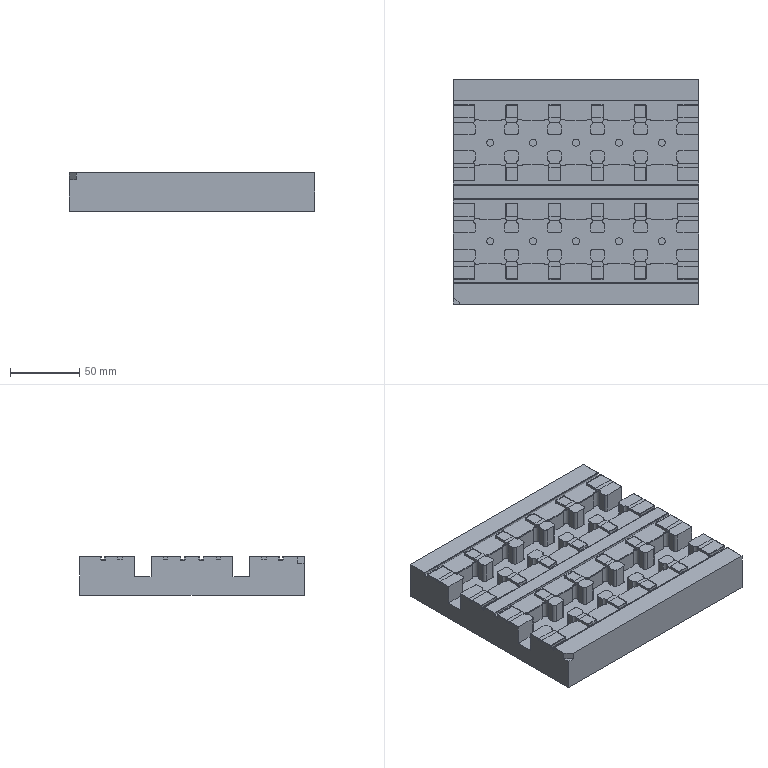NC program | NX | posted by the shop | part box 177 x 162 x 28 mm
Lines 617 to 1664 of 254847:
N4 T10 M06
(D10  D=10. R=0. H=10 ce=0.15 di=0.06)
(MAX_Z=43. MIN_Z=13.56 Time=62.88M)
T05
G00 G90 G54 X96.65 Y35.6 M03 S3000
G43 H10 Z40.
M08
Z29.302
G01 Z27.802 F2000.
X93.4
Y34.75
X74.25
G03 X67.1 Y27.6 I0.0 J-7.15
G01 Y24.98
X56.9
Y27.6
G03 X49.75 Y34.75 I-7.15 J0.0
G01 X43.25
G03 X36.1 Y27.6 I0.0 J-7.15
G01 Y24.98
X25.9
Y27.6
G03 X18.75 Y34.75 I-7.15 J0.0
G01 X12.25
G03 X5.1 Y27.6 I0.0 J-7.15
G01 Y24.98
X-5.1
Y27.6
G03 X-12.25 Y34.75 I-7.15 J0.0
G01 X-18.75
G03 X-25.9 Y27.6 I0.0 J-7.15
G01 Y24.98
X-36.1
Y27.6
G03 X-43.25 Y34.75 I-7.15 J0.0
G01 X-49.75
G03 X-56.9 Y27.6 I0.0 J-7.15
G01 Y24.98
X-67.1
Y27.6
G03 X-74.25 Y34.75 I-7.15 J0.0
G01 X-93.4
Y36.45
X-74.25
G03 X-67.1 Y43.6 I0.0 J7.15
G01 Y46.22
X-56.9
Y43.6
G03 X-55.287 Y39.077 I7.15 J0.0
G02 X-55.062 Y38.444 I-.774 J-.633
X-55.402 Y37.693 I-1. J0.0
G01 X-59.214 Y34.344
G03 X-59.38 Y34.156 I.66 J-.751
X-61.111 Y30.178 I9.63 J-6.556
G02 X-61.989 Y29.479 I-.877 J.202
G01 X-62.015 Y29.48
G02 X-62.889 Y30.178 I.003 J.9
G03 X-65.227 Y34.97 I-11.361 J-2.578
G02 X-65.451 Y35.6 I.777 J.63
X-65.227 Y36.23 I1. J0.0
G03 X-62.889 Y41.022 I-9.023 J7.37
G02 X-62.011 Y41.721 I.877 J-.202
G01 X-61.985 Y41.72
G02 X-61.111 Y41.022 I-.003 J-.9
G03 X-60.428 Y38.941 I11.361 J2.578
X-59.511 Y38.341 I.916 J.4
X-59.177 Y38.398 I0.0 J1.
G01 X-56.397 Y39.386
G02 X-56.062 Y39.444 I.335 J-.942
X-55.287 Y39.077 I0.0 J-1.
G03 X-49.75 Y36.45 I5.537 J4.523
G01 X-43.25
G03 X-36.1 Y43.6 I0.0 J7.15
G01 Y46.22
X-25.9
Y43.6
G03 X-24.287 Y39.077 I7.15 J0.0
G02 X-24.062 Y38.444 I-.774 J-.633
X-24.402 Y37.693 I-1. J0.0
G01 X-28.214 Y34.344
G03 X-28.38 Y34.156 I.66 J-.751
X-30.111 Y30.178 I9.63 J-6.556
G02 X-30.989 Y29.479 I-.877 J.202
G01 X-31.015 Y29.48
G02 X-31.889 Y30.178 I.003 J.9
G03 X-34.227 Y34.97 I-11.361 J-2.578
G02 X-34.451 Y35.6 I.777 J.63
X-34.227 Y36.23 I1. J0.0
G03 X-31.889 Y41.022 I-9.023 J7.37
G02 X-31.011 Y41.721 I.877 J-.202
G01 X-30.985 Y41.72
G02 X-30.111 Y41.022 I-.003 J-.9
G03 X-29.428 Y38.941 I11.361 J2.578
X-28.511 Y38.341 I.916 J.4
X-28.177 Y38.398 I0.0 J1.
G01 X-25.397 Y39.386
G02 X-25.062 Y39.444 I.335 J-.942
X-24.287 Y39.077 I0.0 J-1.
G03 X-18.75 Y36.45 I5.537 J4.523
G01 X-12.25
G03 X-5.1 Y43.6 I0.0 J7.15
G01 Y46.22
X5.1
Y43.6
G03 X6.713 Y39.077 I7.15 J0.0
G02 X6.938 Y38.444 I-.774 J-.633
X6.598 Y37.693 I-1. J0.0
G01 X2.786 Y34.344
G03 X2.62 Y34.156 I.66 J-.751
X.889 Y30.178 I9.63 J-6.556
G02 X.011 Y29.479 I-.877 J.202
G01 X-.015 Y29.48
G02 X-.889 Y30.178 I.003 J.9
G03 X-3.227 Y34.97 I-11.361 J-2.578
G02 X-3.451 Y35.6 I.777 J.63
X-3.227 Y36.23 I1. J0.0
G03 X-.889 Y41.022 I-9.023 J7.37
G02 X-.011 Y41.721 I.877 J-.202
G01 X.015 Y41.72
G02 X.889 Y41.022 I-.003 J-.9
G03 X1.572 Y38.941 I11.361 J2.578
X2.489 Y38.341 I.916 J.4
X2.823 Y38.398 I0.0 J1.
G01 X5.603 Y39.386
G02 X5.938 Y39.444 I.335 J-.942
X6.713 Y39.077 I0.0 J-1.
G03 X12.25 Y36.45 I5.537 J4.523
G01 X18.75
G03 X25.9 Y43.6 I0.0 J7.15
G01 Y46.22
X36.1
Y43.6
G03 X37.713 Y39.077 I7.15 J0.0
G02 X37.938 Y38.444 I-.774 J-.633
X37.598 Y37.693 I-1. J0.0
G01 X33.786 Y34.344
G03 X33.62 Y34.156 I.66 J-.751
X31.889 Y30.178 I9.63 J-6.556
G02 X31.011 Y29.479 I-.877 J.202
G01 X30.985 Y29.48
G02 X30.111 Y30.178 I.003 J.9
G03 X27.773 Y34.97 I-11.361 J-2.578
G02 X27.549 Y35.6 I.777 J.63
X27.773 Y36.23 I1. J0.0
G03 X30.111 Y41.022 I-9.023 J7.37
G02 X30.989 Y41.721 I.877 J-.202
G01 X31.015 Y41.72
G02 X31.889 Y41.022 I-.003 J-.9
G03 X32.572 Y38.941 I11.361 J2.578
X33.489 Y38.341 I.916 J.4
X33.823 Y38.398 I0.0 J1.
G01 X36.603 Y39.386
G02 X36.938 Y39.444 I.335 J-.942
X37.713 Y39.077 I0.0 J-1.
G03 X43.25 Y36.45 I5.537 J4.523
G01 X49.75
G03 X56.9 Y43.6 I0.0 J7.15
G01 Y46.22
X67.1
Y43.6
G03 X68.713 Y39.077 I7.15 J0.0
G02 X68.938 Y38.444 I-.774 J-.633
X68.598 Y37.693 I-1. J0.0
G01 X64.786 Y34.344
G03 X64.62 Y34.156 I.66 J-.751
X62.889 Y30.178 I9.63 J-6.556
G02 X62.011 Y29.479 I-.877 J.202
G01 X61.985 Y29.48
G02 X61.111 Y30.178 I.003 J.9
G03 X58.773 Y34.97 I-11.361 J-2.578
G02 X58.549 Y35.6 I.777 J.63
X58.773 Y36.23 I1. J0.0
G03 X61.111 Y41.022 I-9.023 J7.37
G02 X61.989 Y41.721 I.877 J-.202
G01 X62.015 Y41.72
G02 X62.889 Y41.022 I-.003 J-.9
G03 X63.572 Y38.941 I11.361 J2.578
X64.489 Y38.341 I.916 J.4
X64.823 Y38.398 I0.0 J1.
G01 X67.603 Y39.386
G02 X67.938 Y39.444 I.335 J-.942
X68.713 Y39.077 I0.0 J-1.
G03 X74.25 Y36.45 I5.537 J4.523
G01 X93.4
Y35.6
Y35.1
X96.65
Z29.302
G00 Y35.6
Z29.104
G01 Z27.604
X93.4
Y34.75
X74.25
G03 X67.1 Y27.6 I0.0 J-7.15
G01 Y24.98
X56.9
Y27.6
G03 X49.75 Y34.75 I-7.15 J0.0
G01 X43.25
G03 X36.1 Y27.6 I0.0 J-7.15
G01 Y24.98
X25.9
Y27.6
G03 X18.75 Y34.75 I-7.15 J0.0
G01 X12.25
G03 X5.1 Y27.6 I0.0 J-7.15
G01 Y24.98
X-5.1
Y27.6
G03 X-12.25 Y34.75 I-7.15 J0.0
G01 X-18.75
G03 X-25.9 Y27.6 I0.0 J-7.15
G01 Y24.98
X-36.1
Y27.6
G03 X-43.25 Y34.75 I-7.15 J0.0
G01 X-49.75
G03 X-56.9 Y27.6 I0.0 J-7.15
G01 Y24.98
X-67.1
Y27.6
G03 X-74.25 Y34.75 I-7.15 J0.0
G01 X-93.4
Y36.45
X-74.25
G03 X-67.1 Y43.6 I0.0 J7.15
G01 Y46.22
X-56.9
Y43.6
G03 X-55.287 Y39.077 I7.15 J0.0
G02 X-55.062 Y38.444 I-.774 J-.633
X-55.402 Y37.693 I-1. J0.0
G01 X-59.214 Y34.344
G03 X-59.38 Y34.156 I.66 J-.751
X-61.111 Y30.178 I9.63 J-6.556
G02 X-61.989 Y29.479 I-.877 J.202
G01 X-62.015 Y29.48
G02 X-62.889 Y30.178 I.003 J.9
G03 X-65.227 Y34.97 I-11.361 J-2.578
G02 X-65.451 Y35.6 I.777 J.63
X-65.227 Y36.23 I1. J0.0
G03 X-62.889 Y41.022 I-9.023 J7.37
G02 X-62.011 Y41.721 I.877 J-.202
G01 X-61.985 Y41.72
G02 X-61.111 Y41.022 I-.003 J-.9
G03 X-60.428 Y38.941 I11.361 J2.578
X-59.511 Y38.341 I.916 J.4
X-59.177 Y38.398 I0.0 J1.
G01 X-56.397 Y39.386
G02 X-56.062 Y39.444 I.335 J-.942
X-55.287 Y39.077 I0.0 J-1.
G03 X-49.75 Y36.45 I5.537 J4.523
G01 X-43.25
G03 X-36.1 Y43.6 I0.0 J7.15
G01 Y46.22
X-25.9
Y43.6
G03 X-24.287 Y39.077 I7.15 J0.0
G02 X-24.062 Y38.444 I-.774 J-.633
X-24.402 Y37.693 I-1. J0.0
G01 X-28.214 Y34.344
G03 X-28.38 Y34.156 I.66 J-.751
X-30.111 Y30.178 I9.63 J-6.556
G02 X-30.989 Y29.479 I-.877 J.202
G01 X-31.015 Y29.48
G02 X-31.889 Y30.178 I.003 J.9
G03 X-34.227 Y34.97 I-11.361 J-2.578
G02 X-34.451 Y35.6 I.777 J.63
X-34.227 Y36.23 I1. J0.0
G03 X-31.889 Y41.022 I-9.023 J7.37
G02 X-31.011 Y41.721 I.877 J-.202
G01 X-30.985 Y41.72
G02 X-30.111 Y41.022 I-.003 J-.9
G03 X-29.428 Y38.941 I11.361 J2.578
X-28.511 Y38.341 I.916 J.4
X-28.177 Y38.398 I0.0 J1.
G01 X-25.397 Y39.386
G02 X-25.062 Y39.444 I.335 J-.942
X-24.287 Y39.077 I0.0 J-1.
G03 X-18.75 Y36.45 I5.537 J4.523
G01 X-12.25
G03 X-5.1 Y43.6 I0.0 J7.15
G01 Y46.22
X5.1
Y43.6
G03 X6.713 Y39.077 I7.15 J0.0
G02 X6.938 Y38.444 I-.774 J-.633
X6.598 Y37.693 I-1. J0.0
G01 X2.786 Y34.344
G03 X2.62 Y34.156 I.66 J-.751
X.889 Y30.178 I9.63 J-6.556
G02 X.011 Y29.479 I-.877 J.202
G01 X-.015 Y29.48
G02 X-.889 Y30.178 I.003 J.9
G03 X-3.227 Y34.97 I-11.361 J-2.578
G02 X-3.451 Y35.6 I.777 J.63
X-3.227 Y36.23 I1. J0.0
G03 X-.889 Y41.022 I-9.023 J7.37
G02 X-.011 Y41.721 I.877 J-.202
G01 X.015 Y41.72
G02 X.889 Y41.022 I-.003 J-.9
G03 X1.572 Y38.941 I11.361 J2.578
X2.489 Y38.341 I.916 J.4
X2.823 Y38.398 I0.0 J1.
G01 X5.603 Y39.386
G02 X5.938 Y39.444 I.335 J-.942
X6.713 Y39.077 I0.0 J-1.
G03 X12.25 Y36.45 I5.537 J4.523
G01 X18.75
G03 X25.9 Y43.6 I0.0 J7.15
G01 Y46.22
X36.1
Y43.6
G03 X37.713 Y39.077 I7.15 J0.0
G02 X37.938 Y38.444 I-.774 J-.633
X37.598 Y37.693 I-1. J0.0
G01 X33.786 Y34.344
G03 X33.62 Y34.156 I.66 J-.751
X31.889 Y30.178 I9.63 J-6.556
G02 X31.011 Y29.479 I-.877 J.202
G01 X30.985 Y29.48
G02 X30.111 Y30.178 I.003 J.9
G03 X27.773 Y34.97 I-11.361 J-2.578
G02 X27.549 Y35.6 I.777 J.63
X27.773 Y36.23 I1. J0.0
G03 X30.111 Y41.022 I-9.023 J7.37
G02 X30.989 Y41.721 I.877 J-.202
G01 X31.015 Y41.72
G02 X31.889 Y41.022 I-.003 J-.9
G03 X32.572 Y38.941 I11.361 J2.578
X33.489 Y38.341 I.916 J.4
X33.823 Y38.398 I0.0 J1.
G01 X36.603 Y39.386
G02 X36.938 Y39.444 I.335 J-.942
X37.713 Y39.077 I0.0 J-1.
G03 X43.25 Y36.45 I5.537 J4.523
G01 X49.75
G03 X56.9 Y43.6 I0.0 J7.15
G01 Y46.22
X67.1
Y43.6
G03 X68.713 Y39.077 I7.15 J0.0
G02 X68.938 Y38.444 I-.774 J-.633
X68.598 Y37.693 I-1. J0.0
G01 X64.786 Y34.344
G03 X64.62 Y34.156 I.66 J-.751
X62.889 Y30.178 I9.63 J-6.556
G02 X62.011 Y29.479 I-.877 J.202
G01 X61.985 Y29.48
G02 X61.111 Y30.178 I.003 J.9
G03 X58.773 Y34.97 I-11.361 J-2.578
G02 X58.549 Y35.6 I.777 J.63
X58.773 Y36.23 I1. J0.0
G03 X61.111 Y41.022 I-9.023 J7.37
G02 X61.989 Y41.721 I.877 J-.202
G01 X62.015 Y41.72
G02 X62.889 Y41.022 I-.003 J-.9
G03 X63.572 Y38.941 I11.361 J2.578
X64.489 Y38.341 I.916 J.4
X64.823 Y38.398 I0.0 J1.
G01 X67.603 Y39.386
G02 X67.938 Y39.444 I.335 J-.942
X68.713 Y39.077 I0.0 J-1.
G03 X74.25 Y36.45 I5.537 J4.523
G01 X93.4
Y35.6
Y35.1
X96.65
Z29.104
G00 Y35.6
Z28.907
G01 Z27.407
X93.4
Y34.75
X74.25
G03 X67.1 Y27.6 I0.0 J-7.15
G01 Y24.98
X56.9
Y27.6
G03 X49.75 Y34.75 I-7.15 J0.0
G01 X43.25
G03 X36.1 Y27.6 I0.0 J-7.15
G01 Y24.98
X25.9
Y27.6
G03 X18.75 Y34.75 I-7.15 J0.0
G01 X12.25
G03 X5.1 Y27.6 I0.0 J-7.15
G01 Y24.98
X-5.1
Y27.6
G03 X-12.25 Y34.75 I-7.15 J0.0
G01 X-18.75
G03 X-25.9 Y27.6 I0.0 J-7.15
G01 Y24.98
X-36.1
Y27.6
G03 X-43.25 Y34.75 I-7.15 J0.0
G01 X-49.75
G03 X-56.9 Y27.6 I0.0 J-7.15
G01 Y24.98
X-67.1
Y27.6
G03 X-74.25 Y34.75 I-7.15 J0.0
G01 X-93.4
Y36.45
X-74.25
G03 X-67.1 Y43.6 I0.0 J7.15
G01 Y46.22
X-56.9
Y43.6
G03 X-55.287 Y39.077 I7.15 J0.0
G02 X-55.062 Y38.444 I-.774 J-.633
X-55.402 Y37.693 I-1. J0.0
G01 X-59.214 Y34.344
G03 X-59.38 Y34.156 I.66 J-.751
X-61.111 Y30.178 I9.63 J-6.556
G02 X-61.989 Y29.479 I-.877 J.202
G01 X-62.015 Y29.48
G02 X-62.889 Y30.178 I.003 J.9
G03 X-65.227 Y34.97 I-11.361 J-2.578
G02 X-65.451 Y35.6 I.777 J.63
X-65.227 Y36.23 I1. J0.0
G03 X-62.889 Y41.022 I-9.023 J7.37
G02 X-62.011 Y41.721 I.877 J-.202
G01 X-61.985 Y41.72
G02 X-61.111 Y41.022 I-.003 J-.9
G03 X-60.428 Y38.941 I11.361 J2.578
X-59.511 Y38.341 I.916 J.4
X-59.177 Y38.398 I0.0 J1.
G01 X-56.397 Y39.386
G02 X-56.062 Y39.444 I.335 J-.942
X-55.287 Y39.077 I0.0 J-1.
G03 X-49.75 Y36.45 I5.537 J4.523
G01 X-43.25
G03 X-36.1 Y43.6 I0.0 J7.15
G01 Y46.22
X-25.9
Y43.6
G03 X-24.287 Y39.077 I7.15 J0.0
G02 X-24.062 Y38.444 I-.774 J-.633
X-24.402 Y37.693 I-1. J0.0
G01 X-28.214 Y34.344
G03 X-28.38 Y34.156 I.66 J-.751
X-30.111 Y30.178 I9.63 J-6.556
G02 X-30.989 Y29.479 I-.877 J.202
G01 X-31.015 Y29.48
G02 X-31.889 Y30.178 I.003 J.9
G03 X-34.227 Y34.97 I-11.361 J-2.578
G02 X-34.451 Y35.6 I.777 J.63
X-34.227 Y36.23 I1. J0.0
G03 X-31.889 Y41.022 I-9.023 J7.37
G02 X-31.011 Y41.721 I.877 J-.202
G01 X-30.985 Y41.72
G02 X-30.111 Y41.022 I-.003 J-.9
G03 X-29.428 Y38.941 I11.361 J2.578
X-28.511 Y38.341 I.916 J.4
X-28.177 Y38.398 I0.0 J1.
G01 X-25.397 Y39.386
G02 X-25.062 Y39.444 I.335 J-.942
X-24.287 Y39.077 I0.0 J-1.
G03 X-18.75 Y36.45 I5.537 J4.523
G01 X-12.25
G03 X-5.1 Y43.6 I0.0 J7.15
G01 Y46.22
X5.1
Y43.6
G03 X6.713 Y39.077 I7.15 J0.0
G02 X6.938 Y38.444 I-.774 J-.633
X6.598 Y37.693 I-1. J0.0
G01 X2.786 Y34.344
G03 X2.62 Y34.156 I.66 J-.751
X.889 Y30.178 I9.63 J-6.556
G02 X.011 Y29.479 I-.877 J.202
G01 X-.015 Y29.48
G02 X-.889 Y30.178 I.003 J.9
G03 X-3.227 Y34.97 I-11.361 J-2.578
G02 X-3.451 Y35.6 I.777 J.63
X-3.227 Y36.23 I1. J0.0
G03 X-.889 Y41.022 I-9.023 J7.37
G02 X-.011 Y41.721 I.877 J-.202
G01 X.015 Y41.72
G02 X.889 Y41.022 I-.003 J-.9
G03 X1.572 Y38.941 I11.361 J2.578
X2.489 Y38.341 I.916 J.4
X2.823 Y38.398 I0.0 J1.
G01 X5.603 Y39.386
G02 X5.938 Y39.444 I.335 J-.942
X6.713 Y39.077 I0.0 J-1.
G03 X12.25 Y36.45 I5.537 J4.523
G01 X18.75
G03 X25.9 Y43.6 I0.0 J7.15
G01 Y46.22
X36.1
Y43.6
G03 X37.713 Y39.077 I7.15 J0.0
G02 X37.938 Y38.444 I-.774 J-.633
X37.598 Y37.693 I-1. J0.0
G01 X33.786 Y34.344
G03 X33.62 Y34.156 I.66 J-.751
X31.889 Y30.178 I9.63 J-6.556
G02 X31.011 Y29.479 I-.877 J.202
G01 X30.985 Y29.48
G02 X30.111 Y30.178 I.003 J.9
G03 X27.773 Y34.97 I-11.361 J-2.578
G02 X27.549 Y35.6 I.777 J.63
X27.773 Y36.23 I1. J0.0
G03 X30.111 Y41.022 I-9.023 J7.37
G02 X30.989 Y41.721 I.877 J-.202
G01 X31.015 Y41.72
G02 X31.889 Y41.022 I-.003 J-.9
G03 X32.572 Y38.941 I11.361 J2.578
X33.489 Y38.341 I.916 J.4
X33.823 Y38.398 I0.0 J1.
G01 X36.603 Y39.386
G02 X36.938 Y39.444 I.335 J-.942
X37.713 Y39.077 I0.0 J-1.
G03 X43.25 Y36.45 I5.537 J4.523
G01 X49.75
G03 X56.9 Y43.6 I0.0 J7.15
G01 Y46.22
X67.1
Y43.6
G03 X68.713 Y39.077 I7.15 J0.0
G02 X68.938 Y38.444 I-.774 J-.633
X68.598 Y37.693 I-1. J0.0
G01 X64.786 Y34.344
G03 X64.62 Y34.156 I.66 J-.751
X62.889 Y30.178 I9.63 J-6.556
G02 X62.011 Y29.479 I-.877 J.202
G01 X61.985 Y29.48
G02 X61.111 Y30.178 I.003 J.9
G03 X58.773 Y34.97 I-11.361 J-2.578
G02 X58.549 Y35.6 I.777 J.63
X58.773 Y36.23 I1. J0.0
G03 X61.111 Y41.022 I-9.023 J7.37
G02 X61.989 Y41.721 I.877 J-.202
G01 X62.015 Y41.72
G02 X62.889 Y41.022 I-.003 J-.9
G03 X63.572 Y38.941 I11.361 J2.578
X64.489 Y38.341 I.916 J.4
X64.823 Y38.398 I0.0 J1.
G01 X67.603 Y39.386
G02 X67.938 Y39.444 I.335 J-.942
X68.713 Y39.077 I0.0 J-1.
G03 X74.25 Y36.45 I5.537 J4.523
G01 X93.4
Y35.6
Y35.1
X96.65
Z28.907
G00 Y35.6
Z28.709
G01 Z27.209
X93.4
Y34.75
X74.25
G03 X67.1 Y27.6 I0.0 J-7.15
G01 Y24.98
X56.9
Y27.6
G03 X49.75 Y34.75 I-7.15 J0.0
G01 X43.25
G03 X36.1 Y27.6 I0.0 J-7.15
G01 Y24.98
X25.9
Y27.6
G03 X18.75 Y34.75 I-7.15 J0.0
G01 X12.25
G03 X5.1 Y27.6 I0.0 J-7.15
G01 Y24.98
X-5.1
Y27.6
G03 X-12.25 Y34.75 I-7.15 J0.0
G01 X-18.75
G03 X-25.9 Y27.6 I0.0 J-7.15
G01 Y24.98
X-36.1
Y27.6
G03 X-43.25 Y34.75 I-7.15 J0.0
G01 X-49.75
G03 X-56.9 Y27.6 I0.0 J-7.15
G01 Y24.98
X-67.1
Y27.6
G03 X-74.25 Y34.75 I-7.15 J0.0
G01 X-93.4
Y36.45
X-74.25
G03 X-67.1 Y43.6 I0.0 J7.15
G01 Y46.22
X-56.9
Y43.6
G03 X-55.287 Y39.077 I7.15 J0.0
G02 X-55.062 Y38.444 I-.774 J-.633
X-55.402 Y37.693 I-1. J0.0
G01 X-59.214 Y34.344
G03 X-59.38 Y34.156 I.66 J-.751
X-61.111 Y30.178 I9.63 J-6.556
G02 X-61.989 Y29.479 I-.877 J.202
G01 X-62.015 Y29.48
G02 X-62.889 Y30.178 I.003 J.9
G03 X-65.227 Y34.97 I-11.361 J-2.578
G02 X-65.451 Y35.6 I.777 J.63
X-65.227 Y36.23 I1. J0.0
G03 X-62.889 Y41.022 I-9.023 J7.37
G02 X-62.011 Y41.721 I.877 J-.202
G01 X-61.985 Y41.72
G02 X-61.111 Y41.022 I-.003 J-.9
G03 X-60.428 Y38.941 I11.361 J2.578
X-59.511 Y38.341 I.916 J.4
X-59.177 Y38.398 I0.0 J1.
G01 X-56.397 Y39.386
G02 X-56.062 Y39.444 I.335 J-.942
X-55.287 Y39.077 I0.0 J-1.
G03 X-49.75 Y36.45 I5.537 J4.523
G01 X-43.25
G03 X-36.1 Y43.6 I0.0 J7.15
G01 Y46.22
X-25.9
Y43.6
G03 X-24.287 Y39.077 I7.15 J0.0
G02 X-24.062 Y38.444 I-.774 J-.633
X-24.402 Y37.693 I-1. J0.0
G01 X-28.214 Y34.344
G03 X-28.38 Y34.156 I.66 J-.751
X-30.111 Y30.178 I9.63 J-6.556
G02 X-30.989 Y29.479 I-.877 J.202
G01 X-31.015 Y29.48
G02 X-31.889 Y30.178 I.003 J.9
G03 X-34.227 Y34.97 I-11.361 J-2.578
G02 X-34.451 Y35.6 I.777 J.63
X-34.227 Y36.23 I1. J0.0
G03 X-31.889 Y41.022 I-9.023 J7.37
G02 X-31.011 Y41.721 I.877 J-.202
G01 X-30.985 Y41.72
G02 X-30.111 Y41.022 I-.003 J-.9
G03 X-29.428 Y38.941 I11.361 J2.578
X-28.511 Y38.341 I.916 J.4
X-28.177 Y38.398 I0.0 J1.
G01 X-25.397 Y39.386
G02 X-25.062 Y39.444 I.335 J-.942
X-24.287 Y39.077 I0.0 J-1.
G03 X-18.75 Y36.45 I5.537 J4.523
G01 X-12.25
G03 X-5.1 Y43.6 I0.0 J7.15
G01 Y46.22
X5.1
Y43.6
G03 X6.713 Y39.077 I7.15 J0.0
G02 X6.938 Y38.444 I-.774 J-.633
X6.598 Y37.693 I-1. J0.0
G01 X2.786 Y34.344
G03 X2.62 Y34.156 I.66 J-.751
X.889 Y30.178 I9.63 J-6.556
G02 X.011 Y29.479 I-.877 J.202
G01 X-.015 Y29.48
G02 X-.889 Y30.178 I.003 J.9
G03 X-3.227 Y34.97 I-11.361 J-2.578
G02 X-3.451 Y35.6 I.777 J.63
X-3.227 Y36.23 I1. J0.0
G03 X-.889 Y41.022 I-9.023 J7.37
G02 X-.011 Y41.721 I.877 J-.202
G01 X.015 Y41.72
G02 X.889 Y41.022 I-.003 J-.9
G03 X1.572 Y38.941 I11.361 J2.578
X2.489 Y38.341 I.916 J.4
X2.823 Y38.398 I0.0 J1.
G01 X5.603 Y39.386
G02 X5.938 Y39.444 I.335 J-.942
X6.713 Y39.077 I0.0 J-1.
G03 X12.25 Y36.45 I5.537 J4.523
G01 X18.75
G03 X25.9 Y43.6 I0.0 J7.15
G01 Y46.22
X36.1
Y43.6
G03 X37.713 Y39.077 I7.15 J0.0
G02 X37.938 Y38.444 I-.774 J-.633
X37.598 Y37.693 I-1. J0.0
G01 X33.786 Y34.344
G03 X33.62 Y34.156 I.66 J-.751
X31.889 Y30.178 I9.63 J-6.556
G02 X31.011 Y29.479 I-.877 J.202
G01 X30.985 Y29.48
G02 X30.111 Y30.178 I.003 J.9
G03 X27.773 Y34.97 I-11.361 J-2.578
G02 X27.549 Y35.6 I.777 J.63
X27.773 Y36.23 I1. J0.0
G03 X30.111 Y41.022 I-9.023 J7.37
G02 X30.989 Y41.721 I.877 J-.202
G01 X31.015 Y41.72
G02 X31.889 Y41.022 I-.003 J-.9
G03 X32.572 Y38.941 I11.361 J2.578
X33.489 Y38.341 I.916 J.4
X33.823 Y38.398 I0.0 J1.
G01 X36.603 Y39.386
G02 X36.938 Y39.444 I.335 J-.942
X37.713 Y39.077 I0.0 J-1.
G03 X43.25 Y36.45 I5.537 J4.523
G01 X49.75
G03 X56.9 Y43.6 I0.0 J7.15
G01 Y46.22
X67.1
Y43.6
G03 X68.713 Y39.077 I7.15 J0.0
G02 X68.938 Y38.444 I-.774 J-.633
X68.598 Y37.693 I-1. J0.0
G01 X64.786 Y34.344
G03 X64.62 Y34.156 I.66 J-.751
X62.889 Y30.178 I9.63 J-6.556
G02 X62.011 Y29.479 I-.877 J.202
G01 X61.985 Y29.48
G02 X61.111 Y30.178 I.003 J.9
G03 X58.773 Y34.97 I-11.361 J-2.578
G02 X58.549 Y35.6 I.777 J.63
X58.773 Y36.23 I1. J0.0
G03 X61.111 Y41.022 I-9.023 J7.37
G02 X61.989 Y41.721 I.877 J-.202
G01 X62.015 Y41.72
G02 X62.889 Y41.022 I-.003 J-.9
G03 X63.572 Y38.941 I11.361 J2.578
X64.489 Y38.341 I.916 J.4
X64.823 Y38.398 I0.0 J1.
G01 X67.603 Y39.386
G02 X67.938 Y39.444 I.335 J-.942
X68.713 Y39.077 I0.0 J-1.
G03 X74.25 Y36.45 I5.537 J4.523
G01 X93.4
Y35.6
Y35.1
X96.65
Z28.709
G00 Y35.6
Z28.511
G01 Z27.011
X93.4
Y34.75
X74.25
G03 X67.1 Y27.6 I0.0 J-7.15
G01 Y24.98
X56.9
Y27.6
G03 X49.75 Y34.75 I-7.15 J0.0
G01 X43.25
G03 X36.1 Y27.6 I0.0 J-7.15
G01 Y24.98
X25.9
Y27.6
G03 X18.75 Y34.75 I-7.15 J0.0
G01 X12.25
G03 X5.1 Y27.6 I0.0 J-7.15
G01 Y24.98
X-5.1
Y27.6
G03 X-12.25 Y34.75 I-7.15 J0.0
G01 X-18.75
G03 X-25.9 Y27.6 I0.0 J-7.15
G01 Y24.98
X-36.1
Y27.6
G03 X-43.25 Y34.75 I-7.15 J0.0
G01 X-49.75
G03 X-56.9 Y27.6 I0.0 J-7.15
G01 Y24.98
X-67.1
Y27.6
G03 X-74.25 Y34.75 I-7.15 J0.0
G01 X-93.4
Y36.45
X-74.25
G03 X-67.1 Y43.6 I0.0 J7.15
G01 Y46.22
X-56.9
Y43.6
G03 X-55.287 Y39.077 I7.15 J0.0
G02 X-55.062 Y38.444 I-.774 J-.633
X-55.402 Y37.693 I-1. J0.0
G01 X-59.214 Y34.344
G03 X-59.38 Y34.156 I.66 J-.751
X-61.111 Y30.178 I9.63 J-6.556
G02 X-61.989 Y29.479 I-.877 J.202
G01 X-62.015 Y29.48
G02 X-62.889 Y30.178 I.003 J.9
G03 X-65.227 Y34.97 I-11.361 J-2.578
G02 X-65.451 Y35.6 I.777 J.63
X-65.227 Y36.23 I1. J0.0
G03 X-62.889 Y41.022 I-9.023 J7.37
G02 X-62.011 Y41.721 I.877 J-.202
G01 X-61.985 Y41.72
G02 X-61.111 Y41.022 I-.003 J-.9
G03 X-60.428 Y38.941 I11.361 J2.578
X-59.511 Y38.341 I.916 J.4
X-59.177 Y38.398 I0.0 J1.
G01 X-56.397 Y39.386
G02 X-56.062 Y39.444 I.335 J-.942
X-55.287 Y39.077 I0.0 J-1.
G03 X-49.75 Y36.45 I5.537 J4.523
G01 X-43.25
G03 X-36.1 Y43.6 I0.0 J7.15
G01 Y46.22
X-25.9
Y43.6
G03 X-24.287 Y39.077 I7.15 J0.0
G02 X-24.062 Y38.444 I-.774 J-.633
X-24.402 Y37.693 I-1. J0.0
G01 X-28.214 Y34.344
G03 X-28.38 Y34.156 I.66 J-.751
X-30.111 Y30.178 I9.63 J-6.556
G02 X-30.989 Y29.479 I-.877 J.202
G01 X-31.015 Y29.48
G02 X-31.889 Y30.178 I.003 J.9
G03 X-34.227 Y34.97 I-11.361 J-2.578
G02 X-34.451 Y35.6 I.777 J.63
X-34.227 Y36.23 I1. J0.0
G03 X-31.889 Y41.022 I-9.023 J7.37
G02 X-31.011 Y41.721 I.877 J-.202
G01 X-30.985 Y41.72
G02 X-30.111 Y41.022 I-.003 J-.9
G03 X-29.428 Y38.941 I11.361 J2.578
X-28.511 Y38.341 I.916 J.4
X-28.177 Y38.398 I0.0 J1.
G01 X-25.397 Y39.386
G02 X-25.062 Y39.444 I.335 J-.942
X-24.287 Y39.077 I0.0 J-1.
G03 X-18.75 Y36.45 I5.537 J4.523
G01 X-12.25
G03 X-5.1 Y43.6 I0.0 J7.15
G01 Y46.22
X5.1
Y43.6
G03 X6.713 Y39.077 I7.15 J0.0
G02 X6.938 Y38.444 I-.774 J-.633
X6.598 Y37.693 I-1. J0.0
G01 X2.786 Y34.344
G03 X2.62 Y34.156 I.66 J-.751
X.889 Y30.178 I9.63 J-6.556
G02 X.011 Y29.479 I-.877 J.202
G01 X-.015 Y29.48
G02 X-.889 Y30.178 I.003 J.9
G03 X-3.227 Y34.97 I-11.361 J-2.578
G02 X-3.451 Y35.6 I.777 J.63
X-3.227 Y36.23 I1. J0.0
G03 X-.889 Y41.022 I-9.023 J7.37
G02 X-.011 Y41.721 I.877 J-.202
G01 X.015 Y41.72
G02 X.889 Y41.022 I-.003 J-.9
G03 X1.572 Y38.941 I11.361 J2.578
X2.489 Y38.341 I.916 J.4
X2.823 Y38.398 I0.0 J1.
G01 X5.603 Y39.386
G02 X5.938 Y39.444 I.335 J-.942
X6.713 Y39.077 I0.0 J-1.
G03 X12.25 Y36.45 I5.537 J4.523
G01 X18.75
G03 X25.9 Y43.6 I0.0 J7.15
G01 Y46.22
X36.1
Y43.6
G03 X37.713 Y39.077 I7.15 J0.0
G02 X37.938 Y38.444 I-.774 J-.633
X37.598 Y37.693 I-1. J0.0
G01 X33.786 Y34.344
G03 X33.62 Y34.156 I.66 J-.751
X31.889 Y30.178 I9.63 J-6.556
G02 X31.011 Y29.479 I-.877 J.202
G01 X30.985 Y29.48
G02 X30.111 Y30.178 I.003 J.9
G03 X27.773 Y34.97 I-11.361 J-2.578
G02 X27.549 Y35.6 I.777 J.63
X27.773 Y36.23 I1. J0.0
G03 X30.111 Y41.022 I-9.023 J7.37
G02 X30.989 Y41.721 I.877 J-.202
G01 X31.015 Y41.72
G02 X31.889 Y41.022 I-.003 J-.9
G03 X32.572 Y38.941 I11.361 J2.578
X33.489 Y38.341 I.916 J.4
X33.823 Y38.398 I0.0 J1.
G01 X36.603 Y39.386
G02 X36.938 Y39.444 I.335 J-.942
X37.713 Y39.077 I0.0 J-1.
G03 X43.25 Y36.45 I5.537 J4.523
G01 X49.75
G03 X56.9 Y43.6 I0.0 J7.15
G01 Y46.22
X67.1
Y43.6
G03 X68.713 Y39.077 I7.15 J0.0
G02 X68.938 Y38.444 I-.774 J-.633
X68.598 Y37.693 I-1. J0.0
G01 X64.786 Y34.344
G03 X64.62 Y34.156 I.66 J-.751
X62.889 Y30.178 I9.63 J-6.556
G02 X62.011 Y29.479 I-.877 J.202
G01 X61.985 Y29.48
G02 X61.111 Y30.178 I.003 J.9
G03 X58.773 Y34.97 I-11.361 J-2.578
G02 X58.549 Y35.6 I.777 J.63
X58.773 Y36.23 I1. J0.0
G03 X61.111 Y41.022 I-9.023 J7.37
G02 X61.989 Y41.721 I.877 J-.202
G01 X62.015 Y41.72
G02 X62.889 Y41.022 I-.003 J-.9
G03 X63.572 Y38.941 I11.361 J2.578
X64.489 Y38.341 I.916 J.4
X64.823 Y38.398 I0.0 J1.
G01 X67.603 Y39.386
G02 X67.938 Y39.444 I.335 J-.942
X68.713 Y39.077 I0.0 J-1.
G03 X74.25 Y36.45 I5.537 J4.523
G01 X93.4
Y35.6
Y35.1
X96.65
Z28.511
G00 Y35.6
Z28.313
G01 Z26.813
X93.4
Y34.75
X74.25
G03 X67.1 Y27.6 I0.0 J-7.15
G01 Y24.98
X56.9
Y27.6
G03 X49.75 Y34.75 I-7.15 J0.0
G01 X43.25
G03 X36.1 Y27.6 I0.0 J-7.15
G01 Y24.98
X25.9
Y27.6
G03 X18.75 Y34.75 I-7.15 J0.0
G01 X12.25
G03 X5.1 Y27.6 I0.0 J-7.15
G01 Y24.98
X-5.1
Y27.6
G03 X-12.25 Y34.75 I-7.15 J0.0
G01 X-18.75
G03 X-25.9 Y27.6 I0.0 J-7.15
G01 Y24.98
X-36.1
Y27.6
G03 X-43.25 Y34.75 I-7.15 J0.0
G01 X-49.75
G03 X-56.9 Y27.6 I0.0 J-7.15
G01 Y24.98
X-67.1
Y27.6
G03 X-74.25 Y34.75 I-7.15 J0.0
G01 X-93.4
Y36.45
X-74.25
G03 X-67.1 Y43.6 I0.0 J7.15
G01 Y46.22
X-56.9
Y43.6
G03 X-55.287 Y39.077 I7.15 J0.0
G02 X-55.062 Y38.444 I-.774 J-.633
X-55.402 Y37.693 I-1. J0.0
G01 X-59.214 Y34.344
G03 X-59.38 Y34.156 I.66 J-.751
X-61.111 Y30.178 I9.63 J-6.556
G02 X-61.989 Y29.479 I-.877 J.202
G01 X-62.015 Y29.48
G02 X-62.889 Y30.178 I.003 J.9
G03 X-65.227 Y34.97 I-11.361 J-2.578
G02 X-65.451 Y35.6 I.777 J.63
X-65.227 Y36.23 I1. J0.0
G03 X-62.889 Y41.022 I-9.023 J7.37
G02 X-62.011 Y41.721 I.877 J-.202
G01 X-61.985 Y41.72
G02 X-61.111 Y41.022 I-.003 J-.9
G03 X-60.428 Y38.941 I11.361 J2.578
X-59.511 Y38.341 I.916 J.4
X-59.177 Y38.398 I0.0 J1.
G01 X-56.397 Y39.386
G02 X-56.062 Y39.444 I.335 J-.942
X-55.287 Y39.077 I0.0 J-1.
G03 X-49.75 Y36.45 I5.537 J4.523
G01 X-43.25
G03 X-36.1 Y43.6 I0.0 J7.15
G01 Y46.22
X-25.9
Y43.6
G03 X-24.287 Y39.077 I7.15 J0.0
G02 X-24.062 Y38.444 I-.774 J-.633
X-24.402 Y37.693 I-1. J0.0
G01 X-28.214 Y34.344
G03 X-28.38 Y34.156 I.66 J-.751
X-30.111 Y30.178 I9.63 J-6.556
G02 X-30.989 Y29.479 I-.877 J.202
G01 X-31.015 Y29.48
G02 X-31.889 Y30.178 I.003 J.9
G03 X-34.227 Y34.97 I-11.361 J-2.578
G02 X-34.451 Y35.6 I.777 J.63
X-34.227 Y36.23 I1. J0.0
G03 X-31.889 Y41.022 I-9.023 J7.37
G02 X-31.011 Y41.721 I.877 J-.202
G01 X-30.985 Y41.72
G02 X-30.111 Y41.022 I-.003 J-.9
G03 X-29.428 Y38.941 I11.361 J2.578
X-28.511 Y38.341 I.916 J.4
X-28.177 Y38.398 I0.0 J1.
G01 X-25.397 Y39.386
G02 X-25.062 Y39.444 I.335 J-.942
X-24.287 Y39.077 I0.0 J-1.
G03 X-18.75 Y36.45 I5.537 J4.523
G01 X-12.25
G03 X-5.1 Y43.6 I0.0 J7.15
G01 Y46.22
X5.1
Y43.6
G03 X6.713 Y39.077 I7.15 J0.0
G02 X6.938 Y38.444 I-.774 J-.633
X6.598 Y37.693 I-1. J0.0
G01 X2.786 Y34.344
G03 X2.62 Y34.156 I.66 J-.751
X.889 Y30.178 I9.63 J-6.556
G02 X.011 Y29.479 I-.877 J.202
G01 X-.015 Y29.48
G02 X-.889 Y30.178 I.003 J.9
G03 X-3.227 Y34.97 I-11.361 J-2.578
G02 X-3.451 Y35.6 I.777 J.63
X-3.227 Y36.23 I1. J0.0
G03 X-.889 Y41.022 I-9.023 J7.37
G02 X-.011 Y41.721 I.877 J-.202
G01 X.015 Y41.72
G02 X.889 Y41.022 I-.003 J-.9
G03 X1.572 Y38.941 I11.361 J2.578
X2.489 Y38.341 I.916 J.4
X2.823 Y38.398 I0.0 J1.
G01 X5.603 Y39.386
G02 X5.938 Y39.444 I.335 J-.942
X6.713 Y39.077 I0.0 J-1.
G03 X12.25 Y36.45 I5.537 J4.523
G01 X18.75
G03 X25.9 Y43.6 I0.0 J7.15
G01 Y46.22
X36.1
Y43.6
G03 X37.713 Y39.077 I7.15 J0.0
G02 X37.938 Y38.444 I-.774 J-.633
X37.598 Y37.693 I-1. J0.0
G01 X33.786 Y34.344
G03 X33.62 Y34.156 I.66 J-.751
X31.889 Y30.178 I9.63 J-6.556